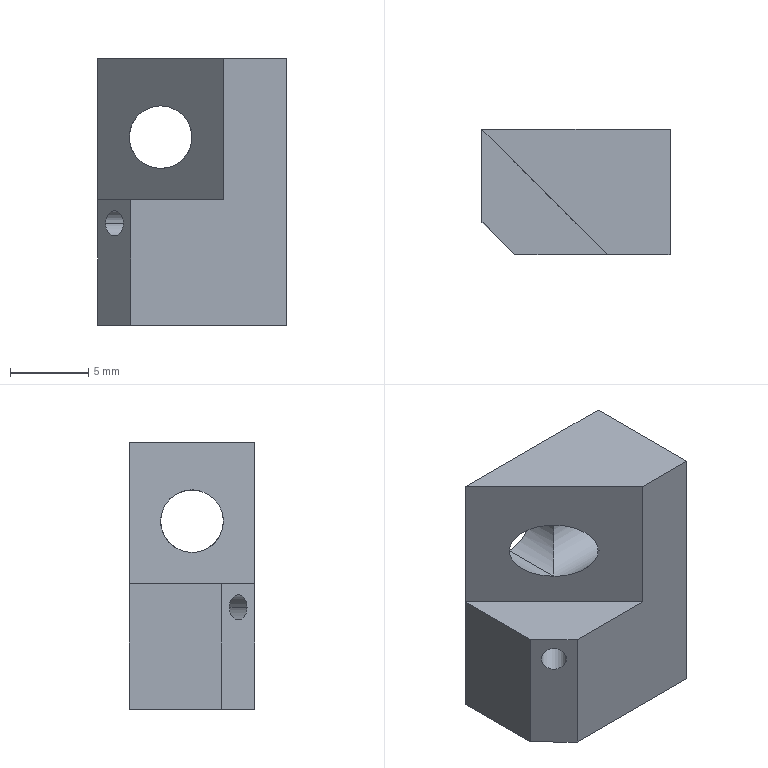Part | NX | 1 solid | 33 faces | box 12 x 8 x 17 mm | volume 1145 mm3 | cylinder 14 | cone 10 | plane 9 | commonest cylinder face diameters 1.6 x6 2 x4 4 x4
STEP:
#1=CARTESIAN_POINT('',(1.,2.5,3.399));
#2=VERTEX_POINT('',#1);
#3=CARTESIAN_POINT('',(-1.,2.5,3.399));
#4=VERTEX_POINT('',#3);
#5=CARTESIAN_POINT('',(0.,2.5,3.399));
#6=DIRECTION('',(0.,0.,-1.));
#7=DIRECTION('',(-1.,0.,0.));
#8=AXIS2_PLACEMENT_3D('',#5,#6,#7);
#9=CIRCLE('',#8,1.);
#10=EDGE_CURVE('',#2,#4,#9,.T.);
#11=ORIENTED_EDGE('',*,*,#10,.F.);
#12=CARTESIAN_POINT('',(1.,2.5,0.));
#13=VERTEX_POINT('',#12);
#14=CARTESIAN_POINT('',(1.,2.5,0.));
#15=DIRECTION('',(0.,0.,-1.));
#16=VECTOR('',#15,1000.);
#17=LINE('',#14,#16);
#18=EDGE_CURVE('',#2,#13,#17,.T.);
#19=ORIENTED_EDGE('',*,*,#18,.T.);
#20=CARTESIAN_POINT('',(-1.,2.5,0.));
#21=VERTEX_POINT('',#20);
#22=CARTESIAN_POINT('',(0.,2.5,0.));
#23=DIRECTION('',(0.,0.,-1.));
#24=DIRECTION('',(-1.,0.,0.));
#25=AXIS2_PLACEMENT_3D('',#22,#23,#24);
#26=CIRCLE('',#25,1.);
#27=EDGE_CURVE('',#13,#21,#26,.T.);
#28=ORIENTED_EDGE('',*,*,#27,.T.);
#29=CARTESIAN_POINT('',(-1.,2.5,0.));
#30=DIRECTION('',(0.,0.,-1.));
#31=VECTOR('',#30,1000.);
#32=LINE('',#29,#31);
#33=EDGE_CURVE('',#4,#21,#32,.T.);
#34=ORIENTED_EDGE('',*,*,#33,.F.);
#35=EDGE_LOOP('',(#11,#19,#28,#34));
#36=FACE_BOUND('',#35,.T.);
#37=CARTESIAN_POINT('',(0.,2.5,0.));
#38=DIRECTION('',(0.,0.,-1.));
#39=DIRECTION('',(1.,0.,0.));
#40=AXIS2_PLACEMENT_3D('',#37,#38,#39);
#41=CYLINDRICAL_SURFACE('',#40,1.);
#42=ADVANCED_FACE('',(#36),#41,.F.);
#43=CARTESIAN_POINT('',(0.,2.5,4.));
#44=VERTEX_POINT('',#43);
#45=CARTESIAN_POINT('',(-1.,2.5,3.399));
#46=DIRECTION('',(-0.8572,0.,-0.515));
#47=VECTOR('',#46,1000.);
#48=LINE('',#45,#47);
#49=EDGE_CURVE('',#44,#4,#48,.T.);
#50=ORIENTED_EDGE('',*,*,#49,.F.);
#51=CARTESIAN_POINT('',(1.,2.5,3.399));
#52=DIRECTION('',(0.8572,0.,-0.515));
#53=VECTOR('',#52,1000.);
#54=LINE('',#51,#53);
#55=EDGE_CURVE('',#44,#2,#54,.T.);
#56=ORIENTED_EDGE('',*,*,#55,.T.);
#57=ORIENTED_EDGE('',*,*,#10,.T.);
#58=EDGE_LOOP('',(#50,#56,#57));
#59=FACE_BOUND('',#58,.T.);
#60=CARTESIAN_POINT('',(0.,2.5,3.399));
#61=DIRECTION('',(0.,0.,-1.));
#62=DIRECTION('',(1.,0.,0.));
#63=AXIS2_PLACEMENT_3D('',#60,#61,#62);
#64=CONICAL_SURFACE('',#63,1.,1.03);
#65=ADVANCED_FACE('',(#59),#64,.F.);
#66=CARTESIAN_POINT('',(1.,-2.5,3.399));
#67=VERTEX_POINT('',#66);
#68=CARTESIAN_POINT('',(-1.,-2.5,3.399));
#69=VERTEX_POINT('',#68);
#70=CARTESIAN_POINT('',(0.,-2.5,3.399));
#71=DIRECTION('',(0.,0.,-1.));
#72=DIRECTION('',(-1.,0.,0.));
#73=AXIS2_PLACEMENT_3D('',#70,#71,#72);
#74=CIRCLE('',#73,1.);
#75=EDGE_CURVE('',#67,#69,#74,.T.);
#76=ORIENTED_EDGE('',*,*,#75,.F.);
#77=CARTESIAN_POINT('',(1.,-2.5,0.));
#78=VERTEX_POINT('',#77);
#79=CARTESIAN_POINT('',(1.,-2.5,0.));
#80=DIRECTION('',(0.,0.,-1.));
#81=VECTOR('',#80,1000.);
#82=LINE('',#79,#81);
#83=EDGE_CURVE('',#67,#78,#82,.T.);
#84=ORIENTED_EDGE('',*,*,#83,.T.);
#85=CARTESIAN_POINT('',(-1.,-2.5,0.));
#86=VERTEX_POINT('',#85);
#87=CARTESIAN_POINT('',(0.,-2.5,0.));
#88=DIRECTION('',(0.,0.,-1.));
#89=DIRECTION('',(-1.,0.,0.));
#90=AXIS2_PLACEMENT_3D('',#87,#88,#89);
#91=CIRCLE('',#90,1.);
#92=EDGE_CURVE('',#78,#86,#91,.T.);
#93=ORIENTED_EDGE('',*,*,#92,.T.);
#94=CARTESIAN_POINT('',(-1.,-2.5,0.));
#95=DIRECTION('',(0.,0.,-1.));
#96=VECTOR('',#95,1000.);
#97=LINE('',#94,#96);
#98=EDGE_CURVE('',#69,#86,#97,.T.);
#99=ORIENTED_EDGE('',*,*,#98,.F.);
#100=EDGE_LOOP('',(#76,#84,#93,#99));
#101=FACE_BOUND('',#100,.T.);
#102=CARTESIAN_POINT('',(0.,-2.5,0.));
#103=DIRECTION('',(0.,0.,-1.));
#104=DIRECTION('',(1.,0.,0.));
#105=AXIS2_PLACEMENT_3D('',#102,#103,#104);
#106=CYLINDRICAL_SURFACE('',#105,1.);
#107=ADVANCED_FACE('',(#101),#106,.F.);
#108=CARTESIAN_POINT('',(0.,-2.5,4.));
#109=VERTEX_POINT('',#108);
#110=CARTESIAN_POINT('',(-1.,-2.5,3.399));
#111=DIRECTION('',(-0.8572,0.,-0.515));
#112=VECTOR('',#111,1000.);
#113=LINE('',#110,#112);
#114=EDGE_CURVE('',#109,#69,#113,.T.);
#115=ORIENTED_EDGE('',*,*,#114,.F.);
#116=CARTESIAN_POINT('',(1.,-2.5,3.399));
#117=DIRECTION('',(0.8572,0.,-0.515));
#118=VECTOR('',#117,1000.);
#119=LINE('',#116,#118);
#120=EDGE_CURVE('',#109,#67,#119,.T.);
#121=ORIENTED_EDGE('',*,*,#120,.T.);
#122=ORIENTED_EDGE('',*,*,#75,.T.);
#123=EDGE_LOOP('',(#115,#121,#122));
#124=FACE_BOUND('',#123,.T.);
#125=CARTESIAN_POINT('',(0.,-2.5,3.399));
#126=DIRECTION('',(0.,0.,-1.));
#127=DIRECTION('',(1.,0.,0.));
#128=AXIS2_PLACEMENT_3D('',#125,#126,#127);
#129=CONICAL_SURFACE('',#128,1.,1.03);
#130=ADVANCED_FACE('',(#124),#129,.F.);
#131=CARTESIAN_POINT('',(-2.179,0.9527,6.5));
#132=VERTEX_POINT('',#131);
#133=CARTESIAN_POINT('',(-1.047,-0.1786,6.5));
#134=VERTEX_POINT('',#133);
#135=CARTESIAN_POINT('',(-1.613,0.3871,6.5));
#136=DIRECTION('',(-0.7071,-0.7071,0.));
#137=DIRECTION('',(0.7071,-0.7071,0.));
#138=AXIS2_PLACEMENT_3D('',#135,#136,#137);
#139=CIRCLE('',#138,0.8);
#140=EDGE_CURVE('',#132,#134,#139,.T.);
#141=ORIENTED_EDGE('',*,*,#140,.F.);
#142=CARTESIAN_POINT('',(-5.516,-2.384,6.5));
#143=VERTEX_POINT('',#142);
#144=CARTESIAN_POINT('',(-5.516,-2.384,6.5));
#145=DIRECTION('',(-0.7071,-0.7071,0.));
#146=VECTOR('',#145,1000.);
#147=LINE('',#144,#146);
#148=EDGE_CURVE('',#132,#143,#147,.T.);
#149=ORIENTED_EDGE('',*,*,#148,.T.);
#150=CARTESIAN_POINT('',(-4.384,-3.516,6.5));
#151=VERTEX_POINT('',#150);
#152=CARTESIAN_POINT('',(-4.95,-2.95,6.5));
#153=DIRECTION('',(-0.7071,-0.7071,0.));
#154=DIRECTION('',(0.7071,-0.7071,0.));
#155=AXIS2_PLACEMENT_3D('',#152,#153,#154);
#156=CIRCLE('',#155,0.8);
#157=EDGE_CURVE('',#143,#151,#156,.T.);
#158=ORIENTED_EDGE('',*,*,#157,.T.);
#159=CARTESIAN_POINT('',(-4.384,-3.516,6.5));
#160=DIRECTION('',(-0.7071,-0.7071,0.));
#161=VECTOR('',#160,1000.);
#162=LINE('',#159,#161);
#163=EDGE_CURVE('',#134,#151,#162,.T.);
#164=ORIENTED_EDGE('',*,*,#163,.F.);
#165=EDGE_LOOP('',(#141,#149,#158,#164));
#166=FACE_BOUND('',#165,.T.);
#167=CARTESIAN_POINT('',(-4.95,-2.95,6.5));
#168=DIRECTION('',(-0.7071,-0.7071,0.));
#169=DIRECTION('',(-0.7071,0.7071,0.));
#170=AXIS2_PLACEMENT_3D('',#167,#168,#169);
#171=CYLINDRICAL_SURFACE('',#170,0.8);
#172=ADVANCED_FACE('',(#166),#171,.F.);
#173=CARTESIAN_POINT('',(-1.273,0.727,6.5));
#174=VERTEX_POINT('',#173);
#175=CARTESIAN_POINT('',(-1.047,-0.1786,6.5));
#176=DIRECTION('',(0.2419,-0.9703,0.));
#177=VECTOR('',#176,1000.);
#178=LINE('',#175,#177);
#179=EDGE_CURVE('',#174,#134,#178,.T.);
#180=ORIENTED_EDGE('',*,*,#179,.F.);
#181=CARTESIAN_POINT('',(-2.179,0.9527,6.5));
#182=DIRECTION('',(-0.9703,0.2419,0.));
#183=VECTOR('',#182,1000.);
#184=LINE('',#181,#183);
#185=EDGE_CURVE('',#174,#132,#184,.T.);
#186=ORIENTED_EDGE('',*,*,#185,.T.);
#187=ORIENTED_EDGE('',*,*,#140,.T.);
#188=EDGE_LOOP('',(#180,#186,#187));
#189=FACE_BOUND('',#188,.T.);
#190=CARTESIAN_POINT('',(-1.613,0.3871,6.5));
#191=DIRECTION('',(-0.7071,-0.7071,0.));
#192=DIRECTION('',(-0.7071,0.7071,0.));
#193=AXIS2_PLACEMENT_3D('',#190,#191,#192);
#194=CONICAL_SURFACE('',#193,0.8,1.03);
#195=ADVANCED_FACE('',(#189),#194,.F.);
#196=CARTESIAN_POINT('',(-2.,0.,10.));
#197=VERTEX_POINT('',#196);
#198=CARTESIAN_POINT('',(-2.,0.,14.));
#199=VERTEX_POINT('',#198);
#200=CARTESIAN_POINT('',(-2.,0.,10.));
#201=CARTESIAN_POINT('',(-6.,4.,10.));
#202=CARTESIAN_POINT('',(-6.,4.,14.));
#203=CARTESIAN_POINT('',(-2.,0.,14.));
#204=(BOUNDED_CURVE()B_SPLINE_CURVE(3,(#200,#201,#202,#203),.UNSPECIFIED.,.F.,.F.)B_SPLINE_CURVE_WITH_KNOTS((4,4),(0.,1.),.PIECEWISE_BEZIER_KNOTS.)CURVE()GEOMETRIC_REPRESENTATION_ITEM()RATIONAL_B_SPLINE_CURVE((1.,0.3333,0.3333,1.))REPRESENTATION_ITEM(''));
#205=EDGE_CURVE('',#197,#199,#204,.T.);
#206=ORIENTED_EDGE('',*,*,#205,.F.);
#207=CARTESIAN_POINT('',(-2.,4.,10.));
#208=VERTEX_POINT('',#207);
#209=CARTESIAN_POINT('',(-2.,-6.,10.));
#210=DIRECTION('',(0.,1.,0.));
#211=VECTOR('',#210,1000.);
#212=LINE('',#209,#211);
#213=EDGE_CURVE('',#197,#208,#212,.T.);
#214=ORIENTED_EDGE('',*,*,#213,.T.);
#215=CARTESIAN_POINT('',(-2.,4.,14.));
#216=VERTEX_POINT('',#215);
#217=CARTESIAN_POINT('',(-2.,4.,12.));
#218=DIRECTION('',(0.,1.,0.));
#219=DIRECTION('',(0.,0.,1.));
#220=AXIS2_PLACEMENT_3D('',#217,#218,#219);
#221=CIRCLE('',#220,2.);
#222=EDGE_CURVE('',#208,#216,#221,.T.);
#223=ORIENTED_EDGE('',*,*,#222,.T.);
#224=CARTESIAN_POINT('',(-2.,-6.,14.));
#225=DIRECTION('',(0.,1.,0.));
#226=VECTOR('',#225,1000.);
#227=LINE('',#224,#226);
#228=EDGE_CURVE('',#199,#216,#227,.T.);
#229=ORIENTED_EDGE('',*,*,#228,.F.);
#230=EDGE_LOOP('',(#206,#214,#223,#229));
#231=FACE_BOUND('',#230,.T.);
#232=CARTESIAN_POINT('',(-2.,-6.,12.));
#233=DIRECTION('',(0.,1.,0.));
#234=DIRECTION('',(0.,0.,-1.));
#235=AXIS2_PLACEMENT_3D('',#232,#233,#234);
#236=CYLINDRICAL_SURFACE('',#235,2.);
#237=ADVANCED_FACE('',(#231),#236,.F.);
#238=CARTESIAN_POINT('',(0.,-2.,12.));
#239=VERTEX_POINT('',#238);
#240=CARTESIAN_POINT('',(0.,-2.,12.));
#241=CARTESIAN_POINT('',(0.,-2.,10.828));
#242=CARTESIAN_POINT('',(-0.8284,-1.172,10.));
#243=CARTESIAN_POINT('',(-2.,0.,10.));
#244=(BOUNDED_CURVE()B_SPLINE_CURVE(3,(#240,#241,#242,#243),.UNSPECIFIED.,.F.,.F.)B_SPLINE_CURVE_WITH_KNOTS((4,4),(0.,1.),.PIECEWISE_BEZIER_KNOTS.)CURVE()GEOMETRIC_REPRESENTATION_ITEM()RATIONAL_B_SPLINE_CURVE((1.,0.8047,0.8047,1.))REPRESENTATION_ITEM(''));
#245=EDGE_CURVE('',#239,#197,#244,.T.);
#246=ORIENTED_EDGE('',*,*,#245,.F.);
#247=CARTESIAN_POINT('',(6.,-2.,12.));
#248=VERTEX_POINT('',#247);
#249=CARTESIAN_POINT('',(-6.,-2.,12.));
#250=DIRECTION('',(1.,0.,0.));
#251=VECTOR('',#250,1000.);
#252=LINE('',#249,#251);
#253=EDGE_CURVE('',#239,#248,#252,.T.);
#254=ORIENTED_EDGE('',*,*,#253,.T.);
#255=CARTESIAN_POINT('',(6.,2.,12.));
#256=VERTEX_POINT('',#255);
#257=CARTESIAN_POINT('',(6.,0.,12.));
#258=DIRECTION('',(1.,0.,0.));
#259=DIRECTION('',(0.,1.,0.));
#260=AXIS2_PLACEMENT_3D('',#257,#258,#259);
#261=CIRCLE('',#260,2.);
#262=EDGE_CURVE('',#248,#256,#261,.T.);
#263=ORIENTED_EDGE('',*,*,#262,.T.);
#264=CARTESIAN_POINT('',(0.,2.,12.));
#265=VERTEX_POINT('',#264);
#266=CARTESIAN_POINT('',(-6.,2.,12.));
#267=DIRECTION('',(1.,0.,0.));
#268=VECTOR('',#267,1000.);
#269=LINE('',#266,#268);
#270=EDGE_CURVE('',#265,#256,#269,.T.);
#271=ORIENTED_EDGE('',*,*,#270,.F.);
#272=CARTESIAN_POINT('',(0.,2.,12.));
#273=CARTESIAN_POINT('',(0.,2.,10.828));
#274=CARTESIAN_POINT('',(-0.8284,1.172,10.));
#275=CARTESIAN_POINT('',(-2.,0.,10.));
#276=(BOUNDED_CURVE()B_SPLINE_CURVE(3,(#272,#273,#274,#275),.UNSPECIFIED.,.F.,.F.)B_SPLINE_CURVE_WITH_KNOTS((4,4),(0.,1.),.PIECEWISE_BEZIER_KNOTS.)CURVE()GEOMETRIC_REPRESENTATION_ITEM()RATIONAL_B_SPLINE_CURVE((1.,0.8047,0.8047,1.))REPRESENTATION_ITEM(''));
#277=EDGE_CURVE('',#265,#197,#276,.T.);
#278=ORIENTED_EDGE('',*,*,#277,.T.);
#279=EDGE_LOOP('',(#246,#254,#263,#271,#278));
#280=FACE_BOUND('',#279,.T.);
#281=CARTESIAN_POINT('',(-6.,0.,12.));
#282=DIRECTION('',(1.,0.,0.));
#283=DIRECTION('',(0.,-1.,0.));
#284=AXIS2_PLACEMENT_3D('',#281,#282,#283);
#285=CYLINDRICAL_SURFACE('',#284,2.);
#286=ADVANCED_FACE('',(#280),#285,.F.);
#287=CARTESIAN_POINT('',(-3.2,0.,4.719));
#288=VERTEX_POINT('',#287);
#289=CARTESIAN_POINT('',(-4.8,0.,4.719));
#290=VERTEX_POINT('',#289);
#291=CARTESIAN_POINT('',(-4.,0.,4.719));
#292=DIRECTION('',(0.,0.,-1.));
#293=DIRECTION('',(-1.,0.,0.));
#294=AXIS2_PLACEMENT_3D('',#291,#292,#293);
#295=CIRCLE('',#294,0.8);
#296=EDGE_CURVE('',#288,#290,#295,.T.);
#297=ORIENTED_EDGE('',*,*,#296,.F.);
#298=CARTESIAN_POINT('',(-3.2,0.,0.));
#299=VERTEX_POINT('',#298);
#300=CARTESIAN_POINT('',(-3.2,0.,0.));
#301=DIRECTION('',(0.,0.,-1.));
#302=VECTOR('',#301,1000.);
#303=LINE('',#300,#302);
#304=EDGE_CURVE('',#288,#299,#303,.T.);
#305=ORIENTED_EDGE('',*,*,#304,.T.);
#306=CARTESIAN_POINT('',(-4.8,0.,0.));
#307=VERTEX_POINT('',#306);
#308=CARTESIAN_POINT('',(-4.,0.,0.));
#309=DIRECTION('',(0.,0.,-1.));
#310=DIRECTION('',(-1.,0.,0.));
#311=AXIS2_PLACEMENT_3D('',#308,#309,#310);
#312=CIRCLE('',#311,0.8);
#313=EDGE_CURVE('',#299,#307,#312,.T.);
#314=ORIENTED_EDGE('',*,*,#313,.T.);
#315=CARTESIAN_POINT('',(-4.8,0.,0.));
#316=DIRECTION('',(0.,0.,-1.));
#317=VECTOR('',#316,1000.);
#318=LINE('',#315,#317);
#319=EDGE_CURVE('',#290,#307,#318,.T.);
#320=ORIENTED_EDGE('',*,*,#319,.F.);
#321=EDGE_LOOP('',(#297,#305,#314,#320));
#322=FACE_BOUND('',#321,.T.);
#323=CARTESIAN_POINT('',(-4.,0.,0.));
#324=DIRECTION('',(0.,0.,-1.));
#325=DIRECTION('',(1.,0.,0.));
#326=AXIS2_PLACEMENT_3D('',#323,#324,#325);
#327=CYLINDRICAL_SURFACE('',#326,0.8);
#328=ADVANCED_FACE('',(#322),#327,.F.);
#329=CARTESIAN_POINT('',(-4.,0.,5.2));
#330=VERTEX_POINT('',#329);
#331=CARTESIAN_POINT('',(-4.8,0.,4.719));
#332=DIRECTION('',(-0.8572,0.,-0.515));
#333=VECTOR('',#332,1000.);
#334=LINE('',#331,#333);
#335=EDGE_CURVE('',#330,#290,#334,.T.);
#336=ORIENTED_EDGE('',*,*,#335,.F.);
#337=CARTESIAN_POINT('',(-3.2,0.,4.719));
#338=DIRECTION('',(0.8572,0.,-0.515));
#339=VECTOR('',#338,1000.);
#340=LINE('',#337,#339);
#341=EDGE_CURVE('',#330,#288,#340,.T.);
#342=ORIENTED_EDGE('',*,*,#341,.T.);
#343=ORIENTED_EDGE('',*,*,#296,.T.);
#344=EDGE_LOOP('',(#336,#342,#343));
#345=FACE_BOUND('',#344,.T.);
#346=CARTESIAN_POINT('',(-4.,0.,4.719));
#347=DIRECTION('',(0.,0.,-1.));
#348=DIRECTION('',(1.,0.,0.));
#349=AXIS2_PLACEMENT_3D('',#346,#347,#348);
#350=CONICAL_SURFACE('',#349,0.8,1.03);
#351=ADVANCED_FACE('',(#345),#350,.F.);
#352=CARTESIAN_POINT('',(4.8,0.,4.719));
#353=VERTEX_POINT('',#352);
#354=CARTESIAN_POINT('',(3.2,0.,4.719));
#355=VERTEX_POINT('',#354);
#356=CARTESIAN_POINT('',(4.,0.,4.719));
#357=DIRECTION('',(0.,0.,-1.));
#358=DIRECTION('',(-1.,0.,0.));
#359=AXIS2_PLACEMENT_3D('',#356,#357,#358);
#360=CIRCLE('',#359,0.8);
#361=EDGE_CURVE('',#353,#355,#360,.T.);
#362=ORIENTED_EDGE('',*,*,#361,.F.);
#363=CARTESIAN_POINT('',(4.8,0.,0.));
#364=VERTEX_POINT('',#363);
#365=CARTESIAN_POINT('',(4.8,0.,0.));
#366=DIRECTION('',(0.,0.,-1.));
#367=VECTOR('',#366,1000.);
#368=LINE('',#365,#367);
#369=EDGE_CURVE('',#353,#364,#368,.T.);
#370=ORIENTED_EDGE('',*,*,#369,.T.);
#371=CARTESIAN_POINT('',(3.2,0.,0.));
#372=VERTEX_POINT('',#371);
#373=CARTESIAN_POINT('',(4.,0.,0.));
#374=DIRECTION('',(0.,0.,-1.));
#375=DIRECTION('',(-1.,0.,0.));
#376=AXIS2_PLACEMENT_3D('',#373,#374,#375);
#377=CIRCLE('',#376,0.8);
#378=EDGE_CURVE('',#364,#372,#377,.T.);
#379=ORIENTED_EDGE('',*,*,#378,.T.);
#380=CARTESIAN_POINT('',(3.2,0.,0.));
#381=DIRECTION('',(0.,0.,-1.));
#382=VECTOR('',#381,1000.);
#383=LINE('',#380,#382);
#384=EDGE_CURVE('',#355,#372,#383,.T.);
#385=ORIENTED_EDGE('',*,*,#384,.F.);
#386=EDGE_LOOP('',(#362,#370,#379,#385));
#387=FACE_BOUND('',#386,.T.);
#388=CARTESIAN_POINT('',(4.,0.,0.));
#389=DIRECTION('',(0.,0.,-1.));
#390=DIRECTION('',(1.,0.,0.));
#391=AXIS2_PLACEMENT_3D('',#388,#389,#390);
#392=CYLINDRICAL_SURFACE('',#391,0.8);
#393=ADVANCED_FACE('',(#387),#392,.F.);
#394=CARTESIAN_POINT('',(4.,0.,5.2));
#395=VERTEX_POINT('',#394);
#396=CARTESIAN_POINT('',(3.2,0.,4.719));
#397=DIRECTION('',(-0.8572,0.,-0.515));
#398=VECTOR('',#397,1000.);
#399=LINE('',#396,#398);
#400=EDGE_CURVE('',#395,#355,#399,.T.);
#401=ORIENTED_EDGE('',*,*,#400,.F.);
#402=CARTESIAN_POINT('',(4.8,0.,4.719));
#403=DIRECTION('',(0.8572,0.,-0.515));
#404=VECTOR('',#403,1000.);
#405=LINE('',#402,#404);
#406=EDGE_CURVE('',#395,#353,#405,.T.);
#407=ORIENTED_EDGE('',*,*,#406,.T.);
#408=ORIENTED_EDGE('',*,*,#361,.T.);
#409=EDGE_LOOP('',(#401,#407,#408));
#410=FACE_BOUND('',#409,.T.);
#411=CARTESIAN_POINT('',(4.,0.,4.719));
#412=DIRECTION('',(0.,0.,-1.));
#413=DIRECTION('',(1.,0.,0.));
#414=AXIS2_PLACEMENT_3D('',#411,#412,#413);
#415=CONICAL_SURFACE('',#414,0.8,1.03);
#416=ADVANCED_FACE('',(#410),#415,.F.);
#417=CARTESIAN_POINT('',(-6.,4.,0.));
#418=VERTEX_POINT('',#417);
#419=CARTESIAN_POINT('',(-6.,-1.9,0.));
#420=VERTEX_POINT('',#419);
#421=CARTESIAN_POINT('',(-6.,4.,0.));
#422=DIRECTION('',(0.,-1.,0.));
#423=VECTOR('',#422,1000.);
#424=LINE('',#421,#423);
#425=EDGE_CURVE('',#418,#420,#424,.T.);
#426=ORIENTED_EDGE('',*,*,#425,.T.);
#427=CARTESIAN_POINT('',(-6.,-1.9,8.));
#428=VERTEX_POINT('',#427);
#429=CARTESIAN_POINT('',(-6.,-1.9,17.));
#430=DIRECTION('',(0.,0.,1.));
#431=VECTOR('',#430,1000.);
#432=LINE('',#429,#431);
#433=EDGE_CURVE('',#420,#428,#432,.T.);
#434=ORIENTED_EDGE('',*,*,#433,.T.);
#435=CARTESIAN_POINT('',(-6.,4.,8.));
#436=VERTEX_POINT('',#435);
#437=CARTESIAN_POINT('',(-6.,4.,8.));
#438=DIRECTION('',(0.,-1.,0.));
#439=VECTOR('',#438,1000.);
#440=LINE('',#437,#439);
#441=EDGE_CURVE('',#436,#428,#440,.T.);
#442=ORIENTED_EDGE('',*,*,#441,.F.);
#443=CARTESIAN_POINT('',(-6.,4.,17.));
#444=DIRECTION('',(0.,0.,-1.));
#445=VECTOR('',#444,1000.);
#446=LINE('',#443,#445);
#447=EDGE_CURVE('',#436,#418,#446,.T.);
#448=ORIENTED_EDGE('',*,*,#447,.T.);
#449=EDGE_LOOP('',(#426,#434,#442,#448));
#450=FACE_BOUND('',#449,.T.);
#451=CARTESIAN_POINT('',(-6.,4.,17.));
#452=DIRECTION('',(1.,0.,0.));
#453=DIRECTION('',(0.,-1.,0.));
#454=AXIS2_PLACEMENT_3D('',#451,#452,#453);
#455=PLANE('',#454);
#456=ADVANCED_FACE('',(#450),#455,.F.);
#457=CARTESIAN_POINT('',(6.,0.,12.));
#458=DIRECTION('',(1.,0.,0.));
#459=DIRECTION('',(0.,1.,0.));
#460=AXIS2_PLACEMENT_3D('',#457,#458,#459);
#461=CIRCLE('',#460,2.);
#462=EDGE_CURVE('',#256,#248,#461,.T.);
#463=ORIENTED_EDGE('',*,*,#462,.F.);
#464=ORIENTED_EDGE('',*,*,#262,.F.);
#465=EDGE_LOOP('',(#463,#464));
#466=FACE_BOUND('',#465,.T.);
#467=CARTESIAN_POINT('',(6.,-4.,0.));
#468=VERTEX_POINT('',#467);
#469=CARTESIAN_POINT('',(6.,4.,0.));
#470=VERTEX_POINT('',#469);
#471=CARTESIAN_POINT('',(6.,4.,0.));
#472=DIRECTION('',(0.,1.,0.));
#473=VECTOR('',#472,1000.);
#474=LINE('',#471,#473);
#475=EDGE_CURVE('',#468,#470,#474,.T.);
#476=ORIENTED_EDGE('',*,*,#475,.T.);
#477=CARTESIAN_POINT('',(6.,4.,17.));
#478=VERTEX_POINT('',#477);
#479=CARTESIAN_POINT('',(6.,4.,17.));
#480=DIRECTION('',(0.,0.,-1.));
#481=VECTOR('',#480,1000.);
#482=LINE('',#479,#481);
#483=EDGE_CURVE('',#478,#470,#482,.T.);
#484=ORIENTED_EDGE('',*,*,#483,.F.);
#485=CARTESIAN_POINT('',(6.,-4.,17.));
#486=VERTEX_POINT('',#485);
#487=CARTESIAN_POINT('',(6.,4.,17.));
#488=DIRECTION('',(0.,1.,0.));
#489=VECTOR('',#488,1000.);
#490=LINE('',#487,#489);
#491=EDGE_CURVE('',#486,#478,#490,.T.);
#492=ORIENTED_EDGE('',*,*,#491,.F.);
#493=CARTESIAN_POINT('',(6.,-4.,17.));
#494=DIRECTION('',(0.,0.,-1.));
#495=VECTOR('',#494,1000.);
#496=LINE('',#493,#495);
#497=EDGE_CURVE('',#486,#468,#496,.T.);
#498=ORIENTED_EDGE('',*,*,#497,.T.);
#499=EDGE_LOOP('',(#476,#484,#492,#498));
#500=FACE_BOUND('',#499,.T.);
#501=CARTESIAN_POINT('',(6.,4.,17.));
#502=DIRECTION('',(-1.,0.,0.));
#503=DIRECTION('',(0.,1.,0.));
#504=AXIS2_PLACEMENT_3D('',#501,#502,#503);
#505=PLANE('',#504);
#506=ADVANCED_FACE('',(#466,#500),#505,.F.);
#507=CARTESIAN_POINT('',(-2.,4.,12.));
#508=DIRECTION('',(0.,1.,0.));
#509=DIRECTION('',(0.,0.,1.));
#510=AXIS2_PLACEMENT_3D('',#507,#508,#509);
#511=CIRCLE('',#510,2.);
#512=EDGE_CURVE('',#216,#208,#511,.T.);
#513=ORIENTED_EDGE('',*,*,#512,.F.);
#514=ORIENTED_EDGE('',*,*,#222,.F.);
#515=EDGE_LOOP('',(#513,#514));
#516=FACE_BOUND('',#515,.T.);
#517=CARTESIAN_POINT('',(-6.,4.,0.));
#518=DIRECTION('',(-1.,0.,0.));
#519=VECTOR('',#518,1000.);
#520=LINE('',#517,#519);
#521=EDGE_CURVE('',#470,#418,#520,.T.);
#522=ORIENTED_EDGE('',*,*,#521,.T.);
#523=ORIENTED_EDGE('',*,*,#447,.F.);
#524=CARTESIAN_POINT('',(-6.,4.,17.));
#525=VERTEX_POINT('',#524);
#526=CARTESIAN_POINT('',(-6.,4.,17.));
#527=DIRECTION('',(0.,0.,-1.));
#528=VECTOR('',#527,1000.);
#529=LINE('',#526,#528);
#530=EDGE_CURVE('',#525,#436,#529,.T.);
#531=ORIENTED_EDGE('',*,*,#530,.F.);
#532=CARTESIAN_POINT('',(-6.,4.,17.));
#533=DIRECTION('',(-1.,0.,0.));
#534=VECTOR('',#533,1000.);
#535=LINE('',#532,#534);
#536=EDGE_CURVE('',#478,#525,#535,.T.);
#537=ORIENTED_EDGE('',*,*,#536,.F.);
#538=ORIENTED_EDGE('',*,*,#483,.T.);
#539=EDGE_LOOP('',(#522,#523,#531,#537,#538));
#540=FACE_BOUND('',#539,.T.);
#541=CARTESIAN_POINT('',(-6.,4.,17.));
#542=DIRECTION('',(0.,-1.,0.));
#543=DIRECTION('',(0.,0.,1.));
#544=AXIS2_PLACEMENT_3D('',#541,#542,#543);
#545=PLANE('',#544);
#546=ADVANCED_FACE('',(#516,#540),#545,.F.);
#547=CARTESIAN_POINT('',(-3.9,-4.,8.));
#548=VERTEX_POINT('',#547);
#549=CARTESIAN_POINT('',(2.,-4.,8.));
#550=VERTEX_POINT('',#549);
#551=CARTESIAN_POINT('',(-6.,-4.,8.));
#552=DIRECTION('',(1.,0.,0.));
#553=VECTOR('',#552,1000.);
#554=LINE('',#551,#553);
#555=EDGE_CURVE('',#548,#550,#554,.T.);
#556=ORIENTED_EDGE('',*,*,#555,.F.);
#557=CARTESIAN_POINT('',(-3.9,-4.,0.));
#558=VERTEX_POINT('',#557);
#559=CARTESIAN_POINT('',(-3.9,-4.,17.));
#560=DIRECTION('',(0.,0.,-1.));
#561=VECTOR('',#560,1000.);
#562=LINE('',#559,#561);
#563=EDGE_CURVE('',#548,#558,#562,.T.);
#564=ORIENTED_EDGE('',*,*,#563,.T.);
#565=CARTESIAN_POINT('',(-6.,-4.,0.));
#566=DIRECTION('',(1.,0.,0.));
#567=VECTOR('',#566,1000.);
#568=LINE('',#565,#567);
#569=EDGE_CURVE('',#558,#468,#568,.T.);
#570=ORIENTED_EDGE('',*,*,#569,.T.);
#571=ORIENTED_EDGE('',*,*,#497,.F.);
#572=CARTESIAN_POINT('',(2.,-4.,17.));
#573=VERTEX_POINT('',#572);
#574=CARTESIAN_POINT('',(-6.,-4.,17.));
#575=DIRECTION('',(1.,0.,0.));
#576=VECTOR('',#575,1000.);
#577=LINE('',#574,#576);
#578=EDGE_CURVE('',#573,#486,#577,.T.);
#579=ORIENTED_EDGE('',*,*,#578,.F.);
#580=CARTESIAN_POINT('',(2.,-4.,8.));
#581=DIRECTION('',(0.,0.,1.));
#582=VECTOR('',#581,1000.);
#583=LINE('',#580,#582);
#584=EDGE_CURVE('',#550,#573,#583,.T.);
#585=ORIENTED_EDGE('',*,*,#584,.F.);
#586=EDGE_LOOP('',(#556,#564,#570,#571,#579,#585));
#587=FACE_BOUND('',#586,.T.);
#588=CARTESIAN_POINT('',(-6.,-4.,17.));
#589=DIRECTION('',(0.,1.,0.));
#590=DIRECTION('',(0.,0.,-1.));
#591=AXIS2_PLACEMENT_3D('',#588,#589,#590);
#592=PLANE('',#591);
#593=ADVANCED_FACE('',(#587),#592,.F.);
#594=CARTESIAN_POINT('',(2.,-4.,17.));
#595=DIRECTION('',(-0.7071,0.7071,0.));
#596=VECTOR('',#595,1000.);
#597=LINE('',#594,#596);
#598=EDGE_CURVE('',#573,#525,#597,.T.);
#599=ORIENTED_EDGE('',*,*,#598,.F.);
#600=ORIENTED_EDGE('',*,*,#578,.T.);
#601=ORIENTED_EDGE('',*,*,#491,.T.);
#602=ORIENTED_EDGE('',*,*,#536,.T.);
#603=EDGE_LOOP('',(#599,#600,#601,#602));
#604=FACE_BOUND('',#603,.T.);
#605=CARTESIAN_POINT('',(0.,0.,17.));
#606=DIRECTION('',(0.,0.,1.));
#607=DIRECTION('',(-1.,0.,0.));
#608=AXIS2_PLACEMENT_3D('',#605,#606,#607);
#609=PLANE('',#608);
#610=ADVANCED_FACE('',(#604),#609,.T.);
#611=CARTESIAN_POINT('',(0.,2.5,0.));
#612=DIRECTION('',(0.,0.,-1.));
#613=DIRECTION('',(-1.,0.,0.));
#614=AXIS2_PLACEMENT_3D('',#611,#612,#613);
#615=CIRCLE('',#614,1.);
#616=EDGE_CURVE('',#21,#13,#615,.T.);
#617=ORIENTED_EDGE('',*,*,#616,.F.);
#618=ORIENTED_EDGE('',*,*,#27,.F.);
#619=EDGE_LOOP('',(#617,#618));
#620=FACE_BOUND('',#619,.T.);
#621=CARTESIAN_POINT('',(0.,-2.5,0.));
#622=DIRECTION('',(0.,0.,-1.));
#623=DIRECTION('',(-1.,0.,0.));
#624=AXIS2_PLACEMENT_3D('',#621,#622,#623);
#625=CIRCLE('',#624,1.);
#626=EDGE_CURVE('',#86,#78,#625,.T.);
#627=ORIENTED_EDGE('',*,*,#626,.F.);
#628=ORIENTED_EDGE('',*,*,#92,.F.);
#629=EDGE_LOOP('',(#627,#628));
#630=FACE_BOUND('',#629,.T.);
#631=CARTESIAN_POINT('',(-4.,0.,0.));
#632=DIRECTION('',(0.,0.,-1.));
#633=DIRECTION('',(-1.,0.,0.));
#634=AXIS2_PLACEMENT_3D('',#631,#632,#633);
#635=CIRCLE('',#634,0.8);
#636=EDGE_CURVE('',#307,#299,#635,.T.);
#637=ORIENTED_EDGE('',*,*,#636,.F.);
#638=ORIENTED_EDGE('',*,*,#313,.F.);
#639=EDGE_LOOP('',(#637,#638));
#640=FACE_BOUND('',#639,.T.);
#641=CARTESIAN_POINT('',(4.,0.,0.));
#642=DIRECTION('',(0.,0.,-1.));
#643=DIRECTION('',(-1.,0.,0.));
#644=AXIS2_PLACEMENT_3D('',#641,#642,#643);
#645=CIRCLE('',#644,0.8);
#646=EDGE_CURVE('',#372,#364,#645,.T.);
#647=ORIENTED_EDGE('',*,*,#646,.F.);
#648=ORIENTED_EDGE('',*,*,#378,.F.);
#649=EDGE_LOOP('',(#647,#648));
#650=FACE_BOUND('',#649,.T.);
#651=ORIENTED_EDGE('',*,*,#569,.F.);
#652=CARTESIAN_POINT('',(-3.9,-4.,0.));
#653=DIRECTION('',(-0.7071,0.7071,0.));
#654=VECTOR('',#653,1000.);
#655=LINE('',#652,#654);
#656=EDGE_CURVE('',#558,#420,#655,.T.);
#657=ORIENTED_EDGE('',*,*,#656,.T.);
#658=ORIENTED_EDGE('',*,*,#425,.F.);
#659=ORIENTED_EDGE('',*,*,#521,.F.);
#660=ORIENTED_EDGE('',*,*,#475,.F.);
#661=EDGE_LOOP('',(#651,#657,#658,#659,#660));
#662=FACE_BOUND('',#661,.T.);
#663=CARTESIAN_POINT('',(0.,0.,0.));
#664=DIRECTION('',(0.,0.,1.));
#665=DIRECTION('',(-1.,0.,0.));
#666=AXIS2_PLACEMENT_3D('',#663,#664,#665);
#667=PLANE('',#666);
#668=ADVANCED_FACE('',(#620,#630,#640,#650,#662),#667,.F.);
#669=ORIENTED_EDGE('',*,*,#205,.T.);
#670=CARTESIAN_POINT('',(-2.,0.,14.));
#671=CARTESIAN_POINT('',(-0.8284,-1.172,14.));
#672=CARTESIAN_POINT('',(0.,-2.,13.172));
#673=CARTESIAN_POINT('',(0.,-2.,12.));
#674=(BOUNDED_CURVE()B_SPLINE_CURVE(3,(#670,#671,#672,#673),.UNSPECIFIED.,.F.,.F.)B_SPLINE_CURVE_WITH_KNOTS((4,4),(0.,1.),.PIECEWISE_BEZIER_KNOTS.)CURVE()GEOMETRIC_REPRESENTATION_ITEM()RATIONAL_B_SPLINE_CURVE((1.,0.8047,0.8047,1.))REPRESENTATION_ITEM(''));
#675=EDGE_CURVE('',#199,#239,#674,.T.);
#676=ORIENTED_EDGE('',*,*,#675,.T.);
#677=ORIENTED_EDGE('',*,*,#245,.T.);
#678=EDGE_LOOP('',(#669,#676,#677));
#679=FACE_BOUND('',#678,.T.);
#680=ORIENTED_EDGE('',*,*,#598,.T.);
#681=ORIENTED_EDGE('',*,*,#530,.T.);
#682=CARTESIAN_POINT('',(2.,-4.,8.));
#683=DIRECTION('',(-0.7071,0.7071,0.));
#684=VECTOR('',#683,1000.);
#685=LINE('',#682,#684);
#686=EDGE_CURVE('',#550,#436,#685,.T.);
#687=ORIENTED_EDGE('',*,*,#686,.F.);
#688=ORIENTED_EDGE('',*,*,#584,.T.);
#689=EDGE_LOOP('',(#680,#681,#687,#688));
#690=FACE_BOUND('',#689,.T.);
#691=CARTESIAN_POINT('',(2.,-4.,8.));
#692=DIRECTION('',(0.7071,0.7071,0.));
#693=DIRECTION('',(0.7071,-0.7071,0.));
#694=AXIS2_PLACEMENT_3D('',#691,#692,#693);
#695=PLANE('',#694);
#696=ADVANCED_FACE('',(#679,#690),#695,.F.);
#697=ORIENTED_EDGE('',*,*,#441,.T.);
#698=CARTESIAN_POINT('',(-3.95,-3.95,8.));
#699=DIRECTION('',(0.7071,-0.7071,0.));
#700=VECTOR('',#699,1000.);
#701=LINE('',#698,#700);
#702=EDGE_CURVE('',#428,#548,#701,.T.);
#703=ORIENTED_EDGE('',*,*,#702,.T.);
#704=ORIENTED_EDGE('',*,*,#555,.T.);
#705=ORIENTED_EDGE('',*,*,#686,.T.);
#706=EDGE_LOOP('',(#697,#703,#704,#705));
#707=FACE_BOUND('',#706,.T.);
#708=CARTESIAN_POINT('',(0.,0.,8.));
#709=DIRECTION('',(0.,0.,1.));
#710=DIRECTION('',(-1.,0.,0.));
#711=AXIS2_PLACEMENT_3D('',#708,#709,#710);
#712=PLANE('',#711);
#713=ADVANCED_FACE('',(#707),#712,.T.);
#714=ORIENTED_EDGE('',*,*,#406,.F.);
#715=ORIENTED_EDGE('',*,*,#400,.T.);
#716=CARTESIAN_POINT('',(4.,0.,4.719));
#717=DIRECTION('',(0.,0.,-1.));
#718=DIRECTION('',(-1.,0.,0.));
#719=AXIS2_PLACEMENT_3D('',#716,#717,#718);
#720=CIRCLE('',#719,0.8);
#721=EDGE_CURVE('',#355,#353,#720,.T.);
#722=ORIENTED_EDGE('',*,*,#721,.T.);
#723=EDGE_LOOP('',(#714,#715,#722));
#724=FACE_BOUND('',#723,.T.);
#725=CARTESIAN_POINT('',(4.,0.,4.719));
#726=DIRECTION('',(0.,0.,-1.));
#727=DIRECTION('',(1.,0.,0.));
#728=AXIS2_PLACEMENT_3D('',#725,#726,#727);
#729=CONICAL_SURFACE('',#728,0.8,1.03);
#730=ADVANCED_FACE('',(#724),#729,.F.);
#731=ORIENTED_EDGE('',*,*,#369,.F.);
#732=ORIENTED_EDGE('',*,*,#721,.F.);
#733=ORIENTED_EDGE('',*,*,#384,.T.);
#734=ORIENTED_EDGE('',*,*,#646,.T.);
#735=EDGE_LOOP('',(#731,#732,#733,#734));
#736=FACE_BOUND('',#735,.T.);
#737=CARTESIAN_POINT('',(4.,0.,0.));
#738=DIRECTION('',(0.,0.,-1.));
#739=DIRECTION('',(1.,0.,0.));
#740=AXIS2_PLACEMENT_3D('',#737,#738,#739);
#741=CYLINDRICAL_SURFACE('',#740,0.8);
#742=ADVANCED_FACE('',(#736),#741,.F.);
#743=ORIENTED_EDGE('',*,*,#341,.F.);
#744=ORIENTED_EDGE('',*,*,#335,.T.);
#745=CARTESIAN_POINT('',(-4.,0.,4.719));
#746=DIRECTION('',(0.,0.,-1.));
#747=DIRECTION('',(-1.,0.,0.));
#748=AXIS2_PLACEMENT_3D('',#745,#746,#747);
#749=CIRCLE('',#748,0.8);
#750=EDGE_CURVE('',#290,#288,#749,.T.);
#751=ORIENTED_EDGE('',*,*,#750,.T.);
#752=EDGE_LOOP('',(#743,#744,#751));
#753=FACE_BOUND('',#752,.T.);
#754=CARTESIAN_POINT('',(-4.,0.,4.719));
#755=DIRECTION('',(0.,0.,-1.));
#756=DIRECTION('',(1.,0.,0.));
#757=AXIS2_PLACEMENT_3D('',#754,#755,#756);
#758=CONICAL_SURFACE('',#757,0.8,1.03);
#759=ADVANCED_FACE('',(#753),#758,.F.);
#760=ORIENTED_EDGE('',*,*,#304,.F.);
#761=ORIENTED_EDGE('',*,*,#750,.F.);
#762=ORIENTED_EDGE('',*,*,#319,.T.);
#763=ORIENTED_EDGE('',*,*,#636,.T.);
#764=EDGE_LOOP('',(#760,#761,#762,#763));
#765=FACE_BOUND('',#764,.T.);
#766=CARTESIAN_POINT('',(-4.,0.,0.));
#767=DIRECTION('',(0.,0.,-1.));
#768=DIRECTION('',(1.,0.,0.));
#769=AXIS2_PLACEMENT_3D('',#766,#767,#768);
#770=CYLINDRICAL_SURFACE('',#769,0.8);
#771=ADVANCED_FACE('',(#765),#770,.F.);
#772=ORIENTED_EDGE('',*,*,#253,.F.);
#773=ORIENTED_EDGE('',*,*,#675,.F.);
#774=CARTESIAN_POINT('',(-2.,0.,14.));
#775=CARTESIAN_POINT('',(-0.8284,1.172,14.));
#776=CARTESIAN_POINT('',(0.,2.,13.172));
#777=CARTESIAN_POINT('',(0.,2.,12.));
#778=(BOUNDED_CURVE()B_SPLINE_CURVE(3,(#774,#775,#776,#777),.UNSPECIFIED.,.F.,.F.)B_SPLINE_CURVE_WITH_KNOTS((4,4),(0.,1.),.PIECEWISE_BEZIER_KNOTS.)CURVE()GEOMETRIC_REPRESENTATION_ITEM()RATIONAL_B_SPLINE_CURVE((1.,0.8047,0.8047,1.))REPRESENTATION_ITEM(''));
#779=EDGE_CURVE('',#199,#265,#778,.T.);
#780=ORIENTED_EDGE('',*,*,#779,.T.);
#781=ORIENTED_EDGE('',*,*,#270,.T.);
#782=ORIENTED_EDGE('',*,*,#462,.T.);
#783=EDGE_LOOP('',(#772,#773,#780,#781,#782));
#784=FACE_BOUND('',#783,.T.);
#785=CARTESIAN_POINT('',(-6.,0.,12.));
#786=DIRECTION('',(1.,0.,0.));
#787=DIRECTION('',(0.,-1.,0.));
#788=AXIS2_PLACEMENT_3D('',#785,#786,#787);
#789=CYLINDRICAL_SURFACE('',#788,2.);
#790=ADVANCED_FACE('',(#784),#789,.F.);
#791=ORIENTED_EDGE('',*,*,#213,.F.);
#792=ORIENTED_EDGE('',*,*,#277,.F.);
#793=ORIENTED_EDGE('',*,*,#779,.F.);
#794=ORIENTED_EDGE('',*,*,#228,.T.);
#795=ORIENTED_EDGE('',*,*,#512,.T.);
#796=EDGE_LOOP('',(#791,#792,#793,#794,#795));
#797=FACE_BOUND('',#796,.T.);
#798=CARTESIAN_POINT('',(-2.,-6.,12.));
#799=DIRECTION('',(0.,1.,0.));
#800=DIRECTION('',(0.,0.,-1.));
#801=AXIS2_PLACEMENT_3D('',#798,#799,#800);
#802=CYLINDRICAL_SURFACE('',#801,2.);
#803=ADVANCED_FACE('',(#797),#802,.F.);
#804=CARTESIAN_POINT('',(-4.95,-2.95,6.5));
#805=DIRECTION('',(-0.7071,-0.7071,0.));
#806=DIRECTION('',(0.7071,-0.7071,0.));
#807=AXIS2_PLACEMENT_3D('',#804,#805,#806);
#808=CIRCLE('',#807,0.8);
#809=EDGE_CURVE('',#151,#143,#808,.T.);
#810=ORIENTED_EDGE('',*,*,#809,.F.);
#811=ORIENTED_EDGE('',*,*,#157,.F.);
#812=EDGE_LOOP('',(#810,#811));
#813=FACE_BOUND('',#812,.T.);
#814=ORIENTED_EDGE('',*,*,#702,.F.);
#815=ORIENTED_EDGE('',*,*,#433,.F.);
#816=ORIENTED_EDGE('',*,*,#656,.F.);
#817=ORIENTED_EDGE('',*,*,#563,.F.);
#818=EDGE_LOOP('',(#814,#815,#816,#817));
#819=FACE_BOUND('',#818,.T.);
#820=CARTESIAN_POINT('',(-3.9,-4.,17.));
#821=DIRECTION('',(0.7071,0.7071,0.));
#822=DIRECTION('',(0.,0.,1.));
#823=AXIS2_PLACEMENT_3D('',#820,#821,#822);
#824=PLANE('',#823);
#825=ADVANCED_FACE('',(#813,#819),#824,.F.);
#826=ORIENTED_EDGE('',*,*,#185,.F.);
#827=ORIENTED_EDGE('',*,*,#179,.T.);
#828=CARTESIAN_POINT('',(-1.613,0.3871,6.5));
#829=DIRECTION('',(-0.7071,-0.7071,0.));
#830=DIRECTION('',(0.7071,-0.7071,0.));
#831=AXIS2_PLACEMENT_3D('',#828,#829,#830);
#832=CIRCLE('',#831,0.8);
#833=EDGE_CURVE('',#134,#132,#832,.T.);
#834=ORIENTED_EDGE('',*,*,#833,.T.);
#835=EDGE_LOOP('',(#826,#827,#834));
#836=FACE_BOUND('',#835,.T.);
#837=CARTESIAN_POINT('',(-1.613,0.3871,6.5));
#838=DIRECTION('',(-0.7071,-0.7071,0.));
#839=DIRECTION('',(-0.7071,0.7071,0.));
#840=AXIS2_PLACEMENT_3D('',#837,#838,#839);
#841=CONICAL_SURFACE('',#840,0.8,1.03);
#842=ADVANCED_FACE('',(#836),#841,.F.);
#843=ORIENTED_EDGE('',*,*,#148,.F.);
#844=ORIENTED_EDGE('',*,*,#833,.F.);
#845=ORIENTED_EDGE('',*,*,#163,.T.);
#846=ORIENTED_EDGE('',*,*,#809,.T.);
#847=EDGE_LOOP('',(#843,#844,#845,#846));
#848=FACE_BOUND('',#847,.T.);
#849=CARTESIAN_POINT('',(-4.95,-2.95,6.5));
#850=DIRECTION('',(-0.7071,-0.7071,0.));
#851=DIRECTION('',(-0.7071,0.7071,0.));
#852=AXIS2_PLACEMENT_3D('',#849,#850,#851);
#853=CYLINDRICAL_SURFACE('',#852,0.8);
#854=ADVANCED_FACE('',(#848),#853,.F.);
#855=ORIENTED_EDGE('',*,*,#120,.F.);
#856=ORIENTED_EDGE('',*,*,#114,.T.);
#857=CARTESIAN_POINT('',(0.,-2.5,3.399));
#858=DIRECTION('',(0.,0.,-1.));
#859=DIRECTION('',(-1.,0.,0.));
#860=AXIS2_PLACEMENT_3D('',#857,#858,#859);
#861=CIRCLE('',#860,1.);
#862=EDGE_CURVE('',#69,#67,#861,.T.);
#863=ORIENTED_EDGE('',*,*,#862,.T.);
#864=EDGE_LOOP('',(#855,#856,#863));
#865=FACE_BOUND('',#864,.T.);
#866=CARTESIAN_POINT('',(0.,-2.5,3.399));
#867=DIRECTION('',(0.,0.,-1.));
#868=DIRECTION('',(1.,0.,0.));
#869=AXIS2_PLACEMENT_3D('',#866,#867,#868);
#870=CONICAL_SURFACE('',#869,1.,1.03);
#871=ADVANCED_FACE('',(#865),#870,.F.);
#872=ORIENTED_EDGE('',*,*,#83,.F.);
#873=ORIENTED_EDGE('',*,*,#862,.F.);
#874=ORIENTED_EDGE('',*,*,#98,.T.);
#875=ORIENTED_EDGE('',*,*,#626,.T.);
#876=EDGE_LOOP('',(#872,#873,#874,#875));
#877=FACE_BOUND('',#876,.T.);
#878=CARTESIAN_POINT('',(0.,-2.5,0.));
#879=DIRECTION('',(0.,0.,-1.));
#880=DIRECTION('',(1.,0.,0.));
#881=AXIS2_PLACEMENT_3D('',#878,#879,#880);
#882=CYLINDRICAL_SURFACE('',#881,1.);
#883=ADVANCED_FACE('',(#877),#882,.F.);
#884=ORIENTED_EDGE('',*,*,#55,.F.);
#885=ORIENTED_EDGE('',*,*,#49,.T.);
#886=CARTESIAN_POINT('',(0.,2.5,3.399));
#887=DIRECTION('',(0.,0.,-1.));
#888=DIRECTION('',(-1.,0.,0.));
#889=AXIS2_PLACEMENT_3D('',#886,#887,#888);
#890=CIRCLE('',#889,1.);
#891=EDGE_CURVE('',#4,#2,#890,.T.);
#892=ORIENTED_EDGE('',*,*,#891,.T.);
#893=EDGE_LOOP('',(#884,#885,#892));
#894=FACE_BOUND('',#893,.T.);
#895=CARTESIAN_POINT('',(0.,2.5,3.399));
#896=DIRECTION('',(0.,0.,-1.));
#897=DIRECTION('',(1.,0.,0.));
#898=AXIS2_PLACEMENT_3D('',#895,#896,#897);
#899=CONICAL_SURFACE('',#898,1.,1.03);
#900=ADVANCED_FACE('',(#894),#899,.F.);
#901=ORIENTED_EDGE('',*,*,#18,.F.);
#902=ORIENTED_EDGE('',*,*,#891,.F.);
#903=ORIENTED_EDGE('',*,*,#33,.T.);
#904=ORIENTED_EDGE('',*,*,#616,.T.);
#905=EDGE_LOOP('',(#901,#902,#903,#904));
#906=FACE_BOUND('',#905,.T.);
#907=CARTESIAN_POINT('',(0.,2.5,0.));
#908=DIRECTION('',(0.,0.,-1.));
#909=DIRECTION('',(1.,0.,0.));
#910=AXIS2_PLACEMENT_3D('',#907,#908,#909);
#911=CYLINDRICAL_SURFACE('',#910,1.);
#912=ADVANCED_FACE('',(#906),#911,.F.);
#913=CLOSED_SHELL('',(#42,#65,#107,#130,#172,#195,#237,#286,#328,#351,#393,#416,#456,#506,#546,#593,#610,#668,#696,#713,#730,#742,#759,#771,#790,#803,#825,#842,#854,#871,#883,#900,#912));
#914=MANIFOLD_SOLID_BREP('',#913);
#915=(LENGTH_UNIT()NAMED_UNIT(*)SI_UNIT(.MILLI.,.METRE.));
#916=UNCERTAINTY_MEASURE_WITH_UNIT(LENGTH_MEASURE(0.00001),#915,'','');
#917=(NAMED_UNIT(*)PLANE_ANGLE_UNIT()SI_UNIT($,.RADIAN.));
#918=(NAMED_UNIT(*)SI_UNIT($,.STERADIAN.)SOLID_ANGLE_UNIT());
#919=(GEOMETRIC_REPRESENTATION_CONTEXT(3)GLOBAL_UNCERTAINTY_ASSIGNED_CONTEXT((#916))GLOBAL_UNIT_ASSIGNED_CONTEXT((#915,#917,#918))REPRESENTATION_CONTEXT('',''));
#920=ADVANCED_BREP_SHAPE_REPRESENTATION('',(#914),#919);